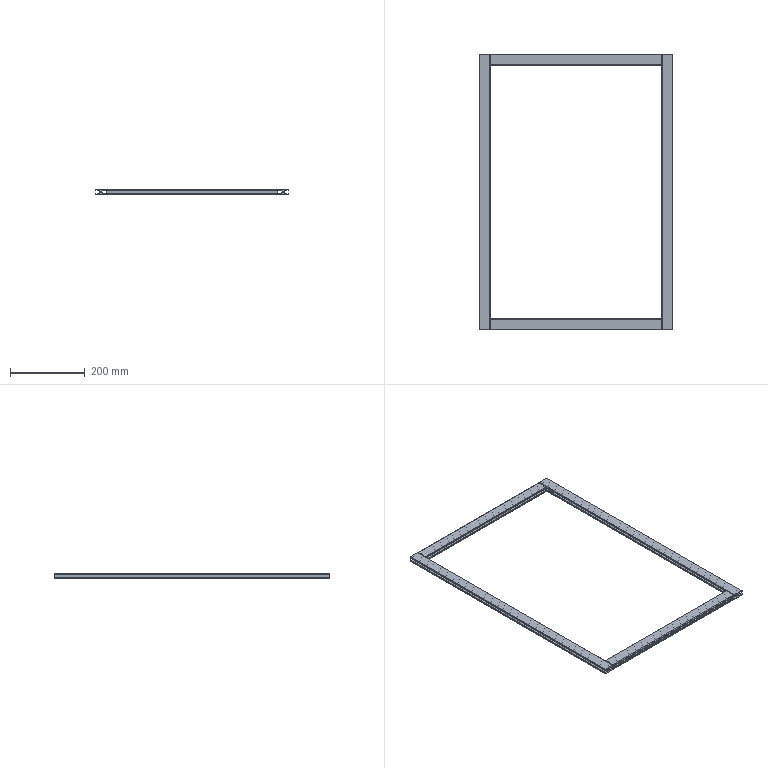Part | STEP file | 001-002-Door frame-2_default<machined> | 4 solids | 144 faces | box 518 x 738 x 15 mm | volume 565549 mm3 | plane 120 | cylinder 24 | commonest cylinder face diameters 3 x16 5 x8